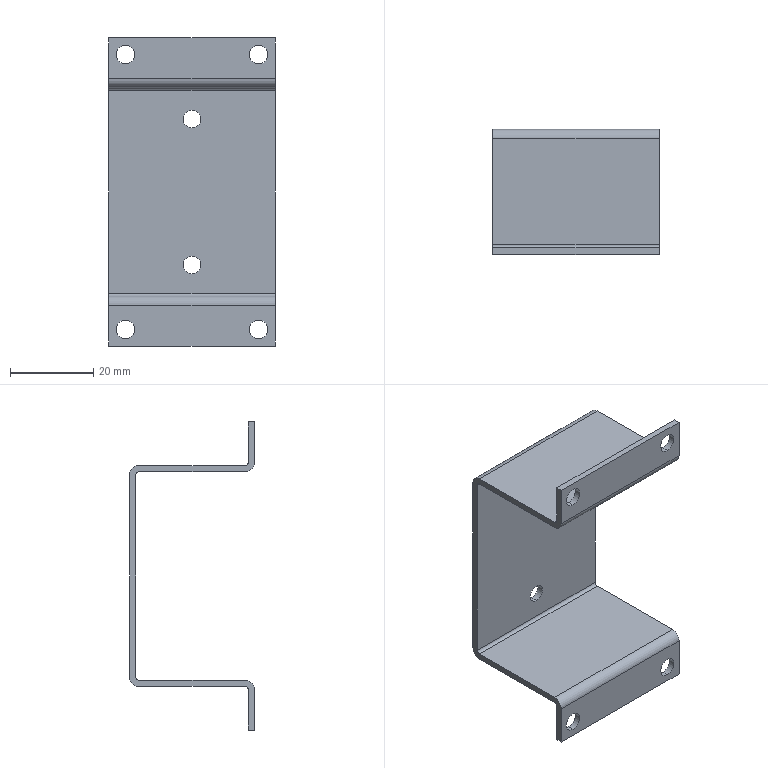Part | SolidWorks | features BaseBody 1 | 1 solid | 34 faces | box 40 x 30 x 74 mm | volume 7570 mm3 | cylinder 20 | plane 14 | commonest cylinder face diameters 4.5 x8 1.473 x4 4.2 x4 4.473 x4
STEP:
#1=CARTESIAN_POINT('',(0.,28.5,19.6));
#2=VERTEX_POINT('',#1);
#3=CARTESIAN_POINT('',(0.,28.5,15.4));
#4=VERTEX_POINT('',#3);
#5=CARTESIAN_POINT('',(0.,28.5,17.5));
#6=DIRECTION('',(0.,-1.,0.));
#7=DIRECTION('',(0.,0.,-1.));
#8=AXIS2_PLACEMENT_3D('',#5,#6,#7);
#9=CIRCLE('',#8,2.1);
#10=EDGE_CURVE('',#2,#4,#9,.T.);
#11=ORIENTED_EDGE('',*,*,#10,.T.);
#12=CARTESIAN_POINT('',(0.,30.,15.4));
#13=VERTEX_POINT('',#12);
#14=CARTESIAN_POINT('',(0.,30.,15.4));
#15=DIRECTION('',(0.,1.,0.));
#16=VECTOR('',#15,1000.);
#17=LINE('',#14,#16);
#18=EDGE_CURVE('',#4,#13,#17,.T.);
#19=ORIENTED_EDGE('',*,*,#18,.T.);
#20=CARTESIAN_POINT('',(0.,30.,19.6));
#21=VERTEX_POINT('',#20);
#22=CARTESIAN_POINT('',(0.,30.,17.5));
#23=DIRECTION('',(0.,1.,0.));
#24=DIRECTION('',(0.,0.,1.));
#25=AXIS2_PLACEMENT_3D('',#22,#23,#24);
#26=CIRCLE('',#25,2.1);
#27=EDGE_CURVE('',#13,#21,#26,.T.);
#28=ORIENTED_EDGE('',*,*,#27,.T.);
#29=CARTESIAN_POINT('',(0.,30.,19.6));
#30=DIRECTION('',(0.,1.,0.));
#31=VECTOR('',#30,1000.);
#32=LINE('',#29,#31);
#33=EDGE_CURVE('',#2,#21,#32,.T.);
#34=ORIENTED_EDGE('',*,*,#33,.F.);
#35=EDGE_LOOP('',(#11,#19,#28,#34));
#36=FACE_OUTER_BOUND('',#35,.T.);
#37=CARTESIAN_POINT('',(0.,30.,17.5));
#38=DIRECTION('',(0.,1.,0.));
#39=DIRECTION('',(0.,0.,1.));
#40=AXIS2_PLACEMENT_3D('',#37,#38,#39);
#41=CYLINDRICAL_SURFACE('',#40,2.1);
#42=ADVANCED_FACE('',(#36),#41,.F.);
#43=CARTESIAN_POINT('',(0.,28.5,-15.4));
#44=VERTEX_POINT('',#43);
#45=CARTESIAN_POINT('',(0.,28.5,-19.6));
#46=VERTEX_POINT('',#45);
#47=CARTESIAN_POINT('',(0.,28.5,-17.5));
#48=DIRECTION('',(0.,-1.,0.));
#49=DIRECTION('',(0.,0.,-1.));
#50=AXIS2_PLACEMENT_3D('',#47,#48,#49);
#51=CIRCLE('',#50,2.1);
#52=EDGE_CURVE('',#44,#46,#51,.T.);
#53=ORIENTED_EDGE('',*,*,#52,.T.);
#54=CARTESIAN_POINT('',(0.,30.,-19.6));
#55=VERTEX_POINT('',#54);
#56=CARTESIAN_POINT('',(0.,30.,-19.6));
#57=DIRECTION('',(0.,1.,0.));
#58=VECTOR('',#57,1000.);
#59=LINE('',#56,#58);
#60=EDGE_CURVE('',#46,#55,#59,.T.);
#61=ORIENTED_EDGE('',*,*,#60,.T.);
#62=CARTESIAN_POINT('',(0.,30.,-15.4));
#63=VERTEX_POINT('',#62);
#64=CARTESIAN_POINT('',(0.,30.,-17.5));
#65=DIRECTION('',(0.,1.,0.));
#66=DIRECTION('',(0.,0.,1.));
#67=AXIS2_PLACEMENT_3D('',#64,#65,#66);
#68=CIRCLE('',#67,2.1);
#69=EDGE_CURVE('',#55,#63,#68,.T.);
#70=ORIENTED_EDGE('',*,*,#69,.T.);
#71=CARTESIAN_POINT('',(0.,30.,-15.4));
#72=DIRECTION('',(0.,1.,0.));
#73=VECTOR('',#72,1000.);
#74=LINE('',#71,#73);
#75=EDGE_CURVE('',#44,#63,#74,.T.);
#76=ORIENTED_EDGE('',*,*,#75,.F.);
#77=EDGE_LOOP('',(#53,#61,#70,#76));
#78=FACE_OUTER_BOUND('',#77,.T.);
#79=CARTESIAN_POINT('',(0.,30.,-17.5));
#80=DIRECTION('',(0.,1.,0.));
#81=DIRECTION('',(0.,0.,1.));
#82=AXIS2_PLACEMENT_3D('',#79,#80,#81);
#83=CYLINDRICAL_SURFACE('',#82,2.1);
#84=ADVANCED_FACE('',(#78),#83,.F.);
#85=CARTESIAN_POINT('',(-16.,0.,30.75));
#86=VERTEX_POINT('',#85);
#87=CARTESIAN_POINT('',(-16.,0.,35.25));
#88=VERTEX_POINT('',#87);
#89=CARTESIAN_POINT('',(-16.,0.,33.));
#90=DIRECTION('',(0.,1.,0.));
#91=DIRECTION('',(0.,0.,-1.));
#92=AXIS2_PLACEMENT_3D('',#89,#90,#91);
#93=CIRCLE('',#92,2.25);
#94=EDGE_CURVE('',#86,#88,#93,.T.);
#95=ORIENTED_EDGE('',*,*,#94,.F.);
#96=CARTESIAN_POINT('',(-16.,1.5,30.75));
#97=VERTEX_POINT('',#96);
#98=CARTESIAN_POINT('',(-16.,0.,30.75));
#99=DIRECTION('',(0.,1.,0.));
#100=VECTOR('',#99,1000.);
#101=LINE('',#98,#100);
#102=EDGE_CURVE('',#86,#97,#101,.T.);
#103=ORIENTED_EDGE('',*,*,#102,.T.);
#104=CARTESIAN_POINT('',(-16.,1.5,35.25));
#105=VERTEX_POINT('',#104);
#106=CARTESIAN_POINT('',(-16.,1.5,33.));
#107=DIRECTION('',(0.,1.,0.));
#108=DIRECTION('',(0.,0.,-1.));
#109=AXIS2_PLACEMENT_3D('',#106,#107,#108);
#110=CIRCLE('',#109,2.25);
#111=EDGE_CURVE('',#97,#105,#110,.T.);
#112=ORIENTED_EDGE('',*,*,#111,.T.);
#113=CARTESIAN_POINT('',(-16.,0.,35.25));
#114=DIRECTION('',(0.,1.,0.));
#115=VECTOR('',#114,1000.);
#116=LINE('',#113,#115);
#117=EDGE_CURVE('',#88,#105,#116,.T.);
#118=ORIENTED_EDGE('',*,*,#117,.F.);
#119=EDGE_LOOP('',(#95,#103,#112,#118));
#120=FACE_OUTER_BOUND('',#119,.T.);
#121=CARTESIAN_POINT('',(-16.,0.,33.));
#122=DIRECTION('',(0.,1.,0.));
#123=DIRECTION('',(0.,0.,1.));
#124=AXIS2_PLACEMENT_3D('',#121,#122,#123);
#125=CYLINDRICAL_SURFACE('',#124,2.25);
#126=ADVANCED_FACE('',(#120),#125,.F.);
#127=CARTESIAN_POINT('',(16.,0.,30.75));
#128=VERTEX_POINT('',#127);
#129=CARTESIAN_POINT('',(16.,0.,35.25));
#130=VERTEX_POINT('',#129);
#131=CARTESIAN_POINT('',(16.,0.,33.));
#132=DIRECTION('',(0.,1.,0.));
#133=DIRECTION('',(0.,0.,1.));
#134=AXIS2_PLACEMENT_3D('',#131,#132,#133);
#135=CIRCLE('',#134,2.25);
#136=EDGE_CURVE('',#128,#130,#135,.T.);
#137=ORIENTED_EDGE('',*,*,#136,.F.);
#138=CARTESIAN_POINT('',(16.,1.5,30.75));
#139=VERTEX_POINT('',#138);
#140=CARTESIAN_POINT('',(16.,0.,30.75));
#141=DIRECTION('',(0.,1.,0.));
#142=VECTOR('',#141,1000.);
#143=LINE('',#140,#142);
#144=EDGE_CURVE('',#128,#139,#143,.T.);
#145=ORIENTED_EDGE('',*,*,#144,.T.);
#146=CARTESIAN_POINT('',(16.,1.5,35.25));
#147=VERTEX_POINT('',#146);
#148=CARTESIAN_POINT('',(16.,1.5,33.));
#149=DIRECTION('',(0.,1.,0.));
#150=DIRECTION('',(0.,0.,1.));
#151=AXIS2_PLACEMENT_3D('',#148,#149,#150);
#152=CIRCLE('',#151,2.25);
#153=EDGE_CURVE('',#139,#147,#152,.T.);
#154=ORIENTED_EDGE('',*,*,#153,.T.);
#155=CARTESIAN_POINT('',(16.,0.,35.25));
#156=DIRECTION('',(0.,1.,0.));
#157=VECTOR('',#156,1000.);
#158=LINE('',#155,#157);
#159=EDGE_CURVE('',#130,#147,#158,.T.);
#160=ORIENTED_EDGE('',*,*,#159,.F.);
#161=EDGE_LOOP('',(#137,#145,#154,#160));
#162=FACE_OUTER_BOUND('',#161,.T.);
#163=CARTESIAN_POINT('',(16.,0.,33.));
#164=DIRECTION('',(0.,1.,0.));
#165=DIRECTION('',(0.,0.,1.));
#166=AXIS2_PLACEMENT_3D('',#163,#164,#165);
#167=CYLINDRICAL_SURFACE('',#166,2.25);
#168=ADVANCED_FACE('',(#162),#167,.F.);
#169=CARTESIAN_POINT('',(16.,0.,-35.25));
#170=VERTEX_POINT('',#169);
#171=CARTESIAN_POINT('',(16.,0.,-30.75));
#172=VERTEX_POINT('',#171);
#173=CARTESIAN_POINT('',(16.,0.,-33.));
#174=DIRECTION('',(0.,1.,0.));
#175=DIRECTION('',(0.,0.,-1.));
#176=AXIS2_PLACEMENT_3D('',#173,#174,#175);
#177=CIRCLE('',#176,2.25);
#178=EDGE_CURVE('',#170,#172,#177,.T.);
#179=ORIENTED_EDGE('',*,*,#178,.F.);
#180=CARTESIAN_POINT('',(16.,1.5,-35.25));
#181=VERTEX_POINT('',#180);
#182=CARTESIAN_POINT('',(16.,0.,-35.25));
#183=DIRECTION('',(0.,1.,0.));
#184=VECTOR('',#183,1000.);
#185=LINE('',#182,#184);
#186=EDGE_CURVE('',#170,#181,#185,.T.);
#187=ORIENTED_EDGE('',*,*,#186,.T.);
#188=CARTESIAN_POINT('',(16.,1.5,-30.75));
#189=VERTEX_POINT('',#188);
#190=CARTESIAN_POINT('',(16.,1.5,-33.));
#191=DIRECTION('',(0.,1.,0.));
#192=DIRECTION('',(0.,0.,-1.));
#193=AXIS2_PLACEMENT_3D('',#190,#191,#192);
#194=CIRCLE('',#193,2.25);
#195=EDGE_CURVE('',#181,#189,#194,.T.);
#196=ORIENTED_EDGE('',*,*,#195,.T.);
#197=CARTESIAN_POINT('',(16.,0.,-30.75));
#198=DIRECTION('',(0.,1.,0.));
#199=VECTOR('',#198,1000.);
#200=LINE('',#197,#199);
#201=EDGE_CURVE('',#172,#189,#200,.T.);
#202=ORIENTED_EDGE('',*,*,#201,.F.);
#203=EDGE_LOOP('',(#179,#187,#196,#202));
#204=FACE_OUTER_BOUND('',#203,.T.);
#205=CARTESIAN_POINT('',(16.,0.,-33.));
#206=DIRECTION('',(0.,1.,0.));
#207=DIRECTION('',(0.,0.,1.));
#208=AXIS2_PLACEMENT_3D('',#205,#206,#207);
#209=CYLINDRICAL_SURFACE('',#208,2.25);
#210=ADVANCED_FACE('',(#204),#209,.F.);
#211=CARTESIAN_POINT('',(-16.,0.,-35.25));
#212=VERTEX_POINT('',#211);
#213=CARTESIAN_POINT('',(-16.,0.,-30.75));
#214=VERTEX_POINT('',#213);
#215=CARTESIAN_POINT('',(-16.,0.,-33.));
#216=DIRECTION('',(0.,1.,0.));
#217=DIRECTION('',(0.,0.,1.));
#218=AXIS2_PLACEMENT_3D('',#215,#216,#217);
#219=CIRCLE('',#218,2.25);
#220=EDGE_CURVE('',#212,#214,#219,.T.);
#221=ORIENTED_EDGE('',*,*,#220,.F.);
#222=CARTESIAN_POINT('',(-16.,1.5,-35.25));
#223=VERTEX_POINT('',#222);
#224=CARTESIAN_POINT('',(-16.,0.,-35.25));
#225=DIRECTION('',(0.,1.,0.));
#226=VECTOR('',#225,1000.);
#227=LINE('',#224,#226);
#228=EDGE_CURVE('',#212,#223,#227,.T.);
#229=ORIENTED_EDGE('',*,*,#228,.T.);
#230=CARTESIAN_POINT('',(-16.,1.5,-30.75));
#231=VERTEX_POINT('',#230);
#232=CARTESIAN_POINT('',(-16.,1.5,-33.));
#233=DIRECTION('',(0.,1.,0.));
#234=DIRECTION('',(0.,0.,1.));
#235=AXIS2_PLACEMENT_3D('',#232,#233,#234);
#236=CIRCLE('',#235,2.25);
#237=EDGE_CURVE('',#223,#231,#236,.T.);
#238=ORIENTED_EDGE('',*,*,#237,.T.);
#239=CARTESIAN_POINT('',(-16.,0.,-30.75));
#240=DIRECTION('',(0.,1.,0.));
#241=VECTOR('',#240,1000.);
#242=LINE('',#239,#241);
#243=EDGE_CURVE('',#214,#231,#242,.T.);
#244=ORIENTED_EDGE('',*,*,#243,.F.);
#245=EDGE_LOOP('',(#221,#229,#238,#244));
#246=FACE_OUTER_BOUND('',#245,.T.);
#247=CARTESIAN_POINT('',(-16.,0.,-33.));
#248=DIRECTION('',(0.,1.,0.));
#249=DIRECTION('',(0.,0.,1.));
#250=AXIS2_PLACEMENT_3D('',#247,#248,#249);
#251=CYLINDRICAL_SURFACE('',#250,2.25);
#252=ADVANCED_FACE('',(#246),#251,.F.);
#253=CARTESIAN_POINT('',(-20.,2.237,26.5));
#254=VERTEX_POINT('',#253);
#255=CARTESIAN_POINT('',(-20.,1.5,27.237));
#256=VERTEX_POINT('',#255);
#257=CARTESIAN_POINT('',(-20.,2.237,27.237));
#258=DIRECTION('',(-1.,0.,0.));
#259=DIRECTION('',(0.,0.,-1.));
#260=AXIS2_PLACEMENT_3D('',#257,#258,#259);
#261=CIRCLE('',#260,0.7366);
#262=EDGE_CURVE('',#254,#256,#261,.T.);
#263=ORIENTED_EDGE('',*,*,#262,.T.);
#264=CARTESIAN_POINT('',(20.,1.5,27.237));
#265=VERTEX_POINT('',#264);
#266=CARTESIAN_POINT('',(20.,1.5,27.237));
#267=DIRECTION('',(-1.,0.,0.));
#268=VECTOR('',#267,1000.);
#269=LINE('',#266,#268);
#270=EDGE_CURVE('',#265,#256,#269,.T.);
#271=ORIENTED_EDGE('',*,*,#270,.F.);
#272=CARTESIAN_POINT('',(20.,2.237,26.5));
#273=VERTEX_POINT('',#272);
#274=CARTESIAN_POINT('',(20.,2.237,27.237));
#275=DIRECTION('',(-1.,0.,0.));
#276=DIRECTION('',(0.,0.,-1.));
#277=AXIS2_PLACEMENT_3D('',#274,#275,#276);
#278=CIRCLE('',#277,0.7366);
#279=EDGE_CURVE('',#273,#265,#278,.T.);
#280=ORIENTED_EDGE('',*,*,#279,.F.);
#281=CARTESIAN_POINT('',(20.,2.237,26.5));
#282=DIRECTION('',(-1.,0.,0.));
#283=VECTOR('',#282,1000.);
#284=LINE('',#281,#283);
#285=EDGE_CURVE('',#273,#254,#284,.T.);
#286=ORIENTED_EDGE('',*,*,#285,.T.);
#287=EDGE_LOOP('',(#263,#271,#280,#286));
#288=FACE_OUTER_BOUND('',#287,.T.);
#289=CARTESIAN_POINT('',(20.,2.237,27.237));
#290=DIRECTION('',(-1.,0.,0.));
#291=DIRECTION('',(0.,0.,1.));
#292=AXIS2_PLACEMENT_3D('',#289,#290,#291);
#293=CYLINDRICAL_SURFACE('',#292,0.7366);
#294=ADVANCED_FACE('',(#288),#293,.F.);
#295=CARTESIAN_POINT('',(-20.,27.763,26.5));
#296=VERTEX_POINT('',#295);
#297=CARTESIAN_POINT('',(-20.,0.,26.5));
#298=DIRECTION('',(0.,-1.,0.));
#299=VECTOR('',#298,1000.);
#300=LINE('',#297,#299);
#301=EDGE_CURVE('',#296,#254,#300,.T.);
#302=ORIENTED_EDGE('',*,*,#301,.T.);
#303=ORIENTED_EDGE('',*,*,#285,.F.);
#304=CARTESIAN_POINT('',(20.,27.763,26.5));
#305=VERTEX_POINT('',#304);
#306=CARTESIAN_POINT('',(20.,0.,26.5));
#307=DIRECTION('',(0.,-1.,0.));
#308=VECTOR('',#307,1000.);
#309=LINE('',#306,#308);
#310=EDGE_CURVE('',#305,#273,#309,.T.);
#311=ORIENTED_EDGE('',*,*,#310,.F.);
#312=CARTESIAN_POINT('',(20.,27.763,26.5));
#313=DIRECTION('',(-1.,0.,0.));
#314=VECTOR('',#313,1000.);
#315=LINE('',#312,#314);
#316=EDGE_CURVE('',#305,#296,#315,.T.);
#317=ORIENTED_EDGE('',*,*,#316,.T.);
#318=EDGE_LOOP('',(#302,#303,#311,#317));
#319=FACE_OUTER_BOUND('',#318,.T.);
#320=CARTESIAN_POINT('',(20.,0.,26.5));
#321=DIRECTION('',(0.,0.,-1.));
#322=DIRECTION('',(0.,-1.,0.));
#323=AXIS2_PLACEMENT_3D('',#320,#321,#322);
#324=PLANE('',#323);
#325=ADVANCED_FACE('',(#319),#324,.F.);
#326=CARTESIAN_POINT('',(-20.,30.,24.263));
#327=VERTEX_POINT('',#326);
#328=CARTESIAN_POINT('',(-20.,27.763,24.263));
#329=DIRECTION('',(1.,0.,0.));
#330=DIRECTION('',(0.,0.,-1.));
#331=AXIS2_PLACEMENT_3D('',#328,#329,#330);
#332=CIRCLE('',#331,2.237);
#333=EDGE_CURVE('',#327,#296,#332,.T.);
#334=ORIENTED_EDGE('',*,*,#333,.T.);
#335=ORIENTED_EDGE('',*,*,#316,.F.);
#336=CARTESIAN_POINT('',(20.,30.,24.263));
#337=VERTEX_POINT('',#336);
#338=CARTESIAN_POINT('',(20.,27.763,24.263));
#339=DIRECTION('',(1.,0.,0.));
#340=DIRECTION('',(0.,0.,-1.));
#341=AXIS2_PLACEMENT_3D('',#338,#339,#340);
#342=CIRCLE('',#341,2.237);
#343=EDGE_CURVE('',#337,#305,#342,.T.);
#344=ORIENTED_EDGE('',*,*,#343,.F.);
#345=CARTESIAN_POINT('',(20.,30.,24.263));
#346=DIRECTION('',(-1.,0.,0.));
#347=VECTOR('',#346,1000.);
#348=LINE('',#345,#347);
#349=EDGE_CURVE('',#337,#327,#348,.T.);
#350=ORIENTED_EDGE('',*,*,#349,.T.);
#351=EDGE_LOOP('',(#334,#335,#344,#350));
#352=FACE_OUTER_BOUND('',#351,.T.);
#353=CARTESIAN_POINT('',(20.,27.763,24.263));
#354=DIRECTION('',(-1.,0.,0.));
#355=DIRECTION('',(0.,0.,1.));
#356=AXIS2_PLACEMENT_3D('',#353,#354,#355);
#357=CYLINDRICAL_SURFACE('',#356,2.237);
#358=ADVANCED_FACE('',(#352),#357,.T.);
#359=CARTESIAN_POINT('',(-20.,27.763,-26.5));
#360=VERTEX_POINT('',#359);
#361=CARTESIAN_POINT('',(-20.,30.,-24.263));
#362=VERTEX_POINT('',#361);
#363=CARTESIAN_POINT('',(-20.,27.763,-24.263));
#364=DIRECTION('',(1.,0.,0.));
#365=DIRECTION('',(0.,0.,-1.));
#366=AXIS2_PLACEMENT_3D('',#363,#364,#365);
#367=CIRCLE('',#366,2.237);
#368=EDGE_CURVE('',#360,#362,#367,.T.);
#369=ORIENTED_EDGE('',*,*,#368,.T.);
#370=CARTESIAN_POINT('',(20.,30.,-24.263));
#371=VERTEX_POINT('',#370);
#372=CARTESIAN_POINT('',(20.,30.,-24.263));
#373=DIRECTION('',(-1.,0.,0.));
#374=VECTOR('',#373,1000.);
#375=LINE('',#372,#374);
#376=EDGE_CURVE('',#371,#362,#375,.T.);
#377=ORIENTED_EDGE('',*,*,#376,.F.);
#378=CARTESIAN_POINT('',(20.,27.763,-26.5));
#379=VERTEX_POINT('',#378);
#380=CARTESIAN_POINT('',(20.,27.763,-24.263));
#381=DIRECTION('',(1.,0.,0.));
#382=DIRECTION('',(0.,0.,-1.));
#383=AXIS2_PLACEMENT_3D('',#380,#381,#382);
#384=CIRCLE('',#383,2.237);
#385=EDGE_CURVE('',#379,#371,#384,.T.);
#386=ORIENTED_EDGE('',*,*,#385,.F.);
#387=CARTESIAN_POINT('',(20.,27.763,-26.5));
#388=DIRECTION('',(-1.,0.,0.));
#389=VECTOR('',#388,1000.);
#390=LINE('',#387,#389);
#391=EDGE_CURVE('',#379,#360,#390,.T.);
#392=ORIENTED_EDGE('',*,*,#391,.T.);
#393=EDGE_LOOP('',(#369,#377,#386,#392));
#394=FACE_OUTER_BOUND('',#393,.T.);
#395=CARTESIAN_POINT('',(20.,27.763,-24.263));
#396=DIRECTION('',(-1.,0.,0.));
#397=DIRECTION('',(0.,0.,1.));
#398=AXIS2_PLACEMENT_3D('',#395,#396,#397);
#399=CYLINDRICAL_SURFACE('',#398,2.237);
#400=ADVANCED_FACE('',(#394),#399,.T.);
#401=CARTESIAN_POINT('',(-20.,2.237,-26.5));
#402=VERTEX_POINT('',#401);
#403=CARTESIAN_POINT('',(-20.,0.,-26.5));
#404=DIRECTION('',(0.,1.,0.));
#405=VECTOR('',#404,1000.);
#406=LINE('',#403,#405);
#407=EDGE_CURVE('',#402,#360,#406,.T.);
#408=ORIENTED_EDGE('',*,*,#407,.T.);
#409=ORIENTED_EDGE('',*,*,#391,.F.);
#410=CARTESIAN_POINT('',(20.,2.237,-26.5));
#411=VERTEX_POINT('',#410);
#412=CARTESIAN_POINT('',(20.,0.,-26.5));
#413=DIRECTION('',(0.,1.,0.));
#414=VECTOR('',#413,1000.);
#415=LINE('',#412,#414);
#416=EDGE_CURVE('',#411,#379,#415,.T.);
#417=ORIENTED_EDGE('',*,*,#416,.F.);
#418=CARTESIAN_POINT('',(20.,2.237,-26.5));
#419=DIRECTION('',(-1.,0.,0.));
#420=VECTOR('',#419,1000.);
#421=LINE('',#418,#420);
#422=EDGE_CURVE('',#411,#402,#421,.T.);
#423=ORIENTED_EDGE('',*,*,#422,.T.);
#424=EDGE_LOOP('',(#408,#409,#417,#423));
#425=FACE_OUTER_BOUND('',#424,.T.);
#426=CARTESIAN_POINT('',(20.,0.,-26.5));
#427=DIRECTION('',(0.,0.,1.));
#428=DIRECTION('',(1.,0.,0.));
#429=AXIS2_PLACEMENT_3D('',#426,#427,#428);
#430=PLANE('',#429);
#431=ADVANCED_FACE('',(#425),#430,.F.);
#432=CARTESIAN_POINT('',(-20.,1.5,-27.237));
#433=VERTEX_POINT('',#432);
#434=CARTESIAN_POINT('',(-20.,2.237,-27.237));
#435=DIRECTION('',(-1.,0.,0.));
#436=DIRECTION('',(0.,0.,-1.));
#437=AXIS2_PLACEMENT_3D('',#434,#435,#436);
#438=CIRCLE('',#437,0.7366);
#439=EDGE_CURVE('',#433,#402,#438,.T.);
#440=ORIENTED_EDGE('',*,*,#439,.T.);
#441=ORIENTED_EDGE('',*,*,#422,.F.);
#442=CARTESIAN_POINT('',(20.,1.5,-27.237));
#443=VERTEX_POINT('',#442);
#444=CARTESIAN_POINT('',(20.,2.237,-27.237));
#445=DIRECTION('',(-1.,0.,0.));
#446=DIRECTION('',(0.,0.,-1.));
#447=AXIS2_PLACEMENT_3D('',#444,#445,#446);
#448=CIRCLE('',#447,0.7366);
#449=EDGE_CURVE('',#443,#411,#448,.T.);
#450=ORIENTED_EDGE('',*,*,#449,.F.);
#451=CARTESIAN_POINT('',(20.,1.5,-27.237));
#452=DIRECTION('',(-1.,0.,0.));
#453=VECTOR('',#452,1000.);
#454=LINE('',#451,#453);
#455=EDGE_CURVE('',#443,#433,#454,.T.);
#456=ORIENTED_EDGE('',*,*,#455,.T.);
#457=EDGE_LOOP('',(#440,#441,#450,#456));
#458=FACE_OUTER_BOUND('',#457,.T.);
#459=CARTESIAN_POINT('',(20.,2.237,-27.237));
#460=DIRECTION('',(-1.,0.,0.));
#461=DIRECTION('',(0.,0.,1.));
#462=AXIS2_PLACEMENT_3D('',#459,#460,#461);
#463=CYLINDRICAL_SURFACE('',#462,0.7366);
#464=ADVANCED_FACE('',(#458),#463,.F.);
#465=CARTESIAN_POINT('',(-16.,1.5,-33.));
#466=DIRECTION('',(0.,1.,0.));
#467=DIRECTION('',(0.,0.,1.));
#468=AXIS2_PLACEMENT_3D('',#465,#466,#467);
#469=CIRCLE('',#468,2.25);
#470=EDGE_CURVE('',#231,#223,#469,.T.);
#471=ORIENTED_EDGE('',*,*,#470,.F.);
#472=ORIENTED_EDGE('',*,*,#237,.F.);
#473=EDGE_LOOP('',(#471,#472));
#474=FACE_BOUND('',#473,.T.);
#475=CARTESIAN_POINT('',(16.,1.5,-33.));
#476=DIRECTION('',(0.,1.,0.));
#477=DIRECTION('',(0.,0.,-1.));
#478=AXIS2_PLACEMENT_3D('',#475,#476,#477);
#479=CIRCLE('',#478,2.25);
#480=EDGE_CURVE('',#189,#181,#479,.T.);
#481=ORIENTED_EDGE('',*,*,#480,.F.);
#482=ORIENTED_EDGE('',*,*,#195,.F.);
#483=EDGE_LOOP('',(#481,#482));
#484=FACE_BOUND('',#483,.T.);
#485=CARTESIAN_POINT('',(-20.,1.5,-37.));
#486=VERTEX_POINT('',#485);
#487=CARTESIAN_POINT('',(-20.,1.5,-37.));
#488=DIRECTION('',(0.,0.,1.));
#489=VECTOR('',#488,1000.);
#490=LINE('',#487,#489);
#491=EDGE_CURVE('',#486,#433,#490,.T.);
#492=ORIENTED_EDGE('',*,*,#491,.T.);
#493=ORIENTED_EDGE('',*,*,#455,.F.);
#494=CARTESIAN_POINT('',(20.,1.5,-37.));
#495=VERTEX_POINT('',#494);
#496=CARTESIAN_POINT('',(20.,1.5,-37.));
#497=DIRECTION('',(0.,0.,1.));
#498=VECTOR('',#497,1000.);
#499=LINE('',#496,#498);
#500=EDGE_CURVE('',#495,#443,#499,.T.);
#501=ORIENTED_EDGE('',*,*,#500,.F.);
#502=CARTESIAN_POINT('',(20.,1.5,-37.));
#503=DIRECTION('',(-1.,0.,0.));
#504=VECTOR('',#503,1000.);
#505=LINE('',#502,#504);
#506=EDGE_CURVE('',#495,#486,#505,.T.);
#507=ORIENTED_EDGE('',*,*,#506,.T.);
#508=EDGE_LOOP('',(#492,#493,#501,#507));
#509=FACE_OUTER_BOUND('',#508,.T.);
#510=CARTESIAN_POINT('',(20.,1.5,-37.));
#511=DIRECTION('',(0.,-1.,0.));
#512=DIRECTION('',(-1.,0.,0.));
#513=AXIS2_PLACEMENT_3D('',#510,#511,#512);
#514=PLANE('',#513);
#515=ADVANCED_FACE('',(#474,#484,#509),#514,.F.);
#516=CARTESIAN_POINT('',(-20.,0.,-37.));
#517=VERTEX_POINT('',#516);
#518=CARTESIAN_POINT('',(-20.,1.5,-37.));
#519=DIRECTION('',(0.,-1.,0.));
#520=VECTOR('',#519,1000.);
#521=LINE('',#518,#520);
#522=EDGE_CURVE('',#486,#517,#521,.T.);
#523=ORIENTED_EDGE('',*,*,#522,.F.);
#524=ORIENTED_EDGE('',*,*,#506,.F.);
#525=CARTESIAN_POINT('',(20.,0.,-37.));
#526=VERTEX_POINT('',#525);
#527=CARTESIAN_POINT('',(20.,1.5,-37.));
#528=DIRECTION('',(0.,-1.,0.));
#529=VECTOR('',#528,1000.);
#530=LINE('',#527,#529);
#531=EDGE_CURVE('',#495,#526,#530,.T.);
#532=ORIENTED_EDGE('',*,*,#531,.T.);
#533=CARTESIAN_POINT('',(20.,0.,-37.));
#534=DIRECTION('',(-1.,0.,0.));
#535=VECTOR('',#534,1000.);
#536=LINE('',#533,#535);
#537=EDGE_CURVE('',#526,#517,#536,.T.);
#538=ORIENTED_EDGE('',*,*,#537,.T.);
#539=EDGE_LOOP('',(#523,#524,#532,#538));
#540=FACE_OUTER_BOUND('',#539,.T.);
#541=CARTESIAN_POINT('',(20.,1.5,-37.));
#542=DIRECTION('',(0.,0.,-1.));
#543=DIRECTION('',(0.,-1.,0.));
#544=AXIS2_PLACEMENT_3D('',#541,#542,#543);
#545=PLANE('',#544);
#546=ADVANCED_FACE('',(#540),#545,.T.);
#547=CARTESIAN_POINT('',(-16.,0.,-33.));
#548=DIRECTION('',(0.,1.,0.));
#549=DIRECTION('',(0.,0.,1.));
#550=AXIS2_PLACEMENT_3D('',#547,#548,#549);
#551=CIRCLE('',#550,2.25);
#552=EDGE_CURVE('',#214,#212,#551,.T.);
#553=ORIENTED_EDGE('',*,*,#552,.T.);
#554=ORIENTED_EDGE('',*,*,#220,.T.);
#555=EDGE_LOOP('',(#553,#554));
#556=FACE_BOUND('',#555,.T.);
#557=CARTESIAN_POINT('',(16.,0.,-33.));
#558=DIRECTION('',(0.,1.,0.));
#559=DIRECTION('',(0.,0.,-1.));
#560=AXIS2_PLACEMENT_3D('',#557,#558,#559);
#561=CIRCLE('',#560,2.25);
#562=EDGE_CURVE('',#172,#170,#561,.T.);
#563=ORIENTED_EDGE('',*,*,#562,.T.);
#564=ORIENTED_EDGE('',*,*,#178,.T.);
#565=EDGE_LOOP('',(#563,#564));
#566=FACE_BOUND('',#565,.T.);
#567=CARTESIAN_POINT('',(-20.,0.,-27.237));
#568=VERTEX_POINT('',#567);
#569=CARTESIAN_POINT('',(-20.,0.,-37.));
#570=DIRECTION('',(0.,0.,1.));
#571=VECTOR('',#570,1000.);
#572=LINE('',#569,#571);
#573=EDGE_CURVE('',#517,#568,#572,.T.);
#574=ORIENTED_EDGE('',*,*,#573,.F.);
#575=ORIENTED_EDGE('',*,*,#537,.F.);
#576=CARTESIAN_POINT('',(20.,0.,-27.237));
#577=VERTEX_POINT('',#576);
#578=CARTESIAN_POINT('',(20.,0.,-37.));
#579=DIRECTION('',(0.,0.,1.));
#580=VECTOR('',#579,1000.);
#581=LINE('',#578,#580);
#582=EDGE_CURVE('',#526,#577,#581,.T.);
#583=ORIENTED_EDGE('',*,*,#582,.T.);
#584=CARTESIAN_POINT('',(20.,0.,-27.237));
#585=DIRECTION('',(-1.,0.,0.));
#586=VECTOR('',#585,1000.);
#587=LINE('',#584,#586);
#588=EDGE_CURVE('',#577,#568,#587,.T.);
#589=ORIENTED_EDGE('',*,*,#588,.T.);
#590=EDGE_LOOP('',(#574,#575,#583,#589));
#591=FACE_OUTER_BOUND('',#590,.T.);
#592=CARTESIAN_POINT('',(20.,0.,-37.));
#593=DIRECTION('',(0.,-1.,0.));
#594=DIRECTION('',(-1.,0.,0.));
#595=AXIS2_PLACEMENT_3D('',#592,#593,#594);
#596=PLANE('',#595);
#597=ADVANCED_FACE('',(#556,#566,#591),#596,.T.);
#598=CARTESIAN_POINT('',(-20.,2.237,-25.));
#599=VERTEX_POINT('',#598);
#600=CARTESIAN_POINT('',(-20.,2.237,-27.237));
#601=DIRECTION('',(-1.,0.,0.));
#602=DIRECTION('',(0.,0.,1.));
#603=AXIS2_PLACEMENT_3D('',#600,#601,#602);
#604=CIRCLE('',#603,2.237);
#605=EDGE_CURVE('',#568,#599,#604,.T.);
#606=ORIENTED_EDGE('',*,*,#605,.F.);
#607=ORIENTED_EDGE('',*,*,#588,.F.);
#608=CARTESIAN_POINT('',(20.,2.237,-25.));
#609=VERTEX_POINT('',#608);
#610=CARTESIAN_POINT('',(20.,2.237,-27.237));
#611=DIRECTION('',(-1.,0.,0.));
#612=DIRECTION('',(0.,0.,1.));
#613=AXIS2_PLACEMENT_3D('',#610,#611,#612);
#614=CIRCLE('',#613,2.237);
#615=EDGE_CURVE('',#577,#609,#614,.T.);
#616=ORIENTED_EDGE('',*,*,#615,.T.);
#617=CARTESIAN_POINT('',(20.,2.237,-25.));
#618=DIRECTION('',(-1.,0.,0.));
#619=VECTOR('',#618,1000.);
#620=LINE('',#617,#619);
#621=EDGE_CURVE('',#609,#599,#620,.T.);
#622=ORIENTED_EDGE('',*,*,#621,.T.);
#623=EDGE_LOOP('',(#606,#607,#616,#622));
#624=FACE_OUTER_BOUND('',#623,.T.);
#625=CARTESIAN_POINT('',(20.,2.237,-27.237));
#626=DIRECTION('',(-1.,0.,0.));
#627=DIRECTION('',(0.,0.,1.));
#628=AXIS2_PLACEMENT_3D('',#625,#626,#627);
#629=CYLINDRICAL_SURFACE('',#628,2.237);
#630=ADVANCED_FACE('',(#624),#629,.T.);
#631=CARTESIAN_POINT('',(-20.,27.763,-25.));
#632=VERTEX_POINT('',#631);
#633=CARTESIAN_POINT('',(-20.,0.,-25.));
#634=DIRECTION('',(0.,1.,0.));
#635=VECTOR('',#634,1000.);
#636=LINE('',#633,#635);
#637=EDGE_CURVE('',#599,#632,#636,.T.);
#638=ORIENTED_EDGE('',*,*,#637,.F.);
#639=ORIENTED_EDGE('',*,*,#621,.F.);
#640=CARTESIAN_POINT('',(20.,27.763,-25.));
#641=VERTEX_POINT('',#640);
#642=CARTESIAN_POINT('',(20.,0.,-25.));
#643=DIRECTION('',(0.,1.,0.));
#644=VECTOR('',#643,1000.);
#645=LINE('',#642,#644);
#646=EDGE_CURVE('',#609,#641,#645,.T.);
#647=ORIENTED_EDGE('',*,*,#646,.T.);
#648=CARTESIAN_POINT('',(20.,27.763,-25.));
#649=DIRECTION('',(-1.,0.,0.));
#650=VECTOR('',#649,1000.);
#651=LINE('',#648,#650);
#652=EDGE_CURVE('',#641,#632,#651,.T.);
#653=ORIENTED_EDGE('',*,*,#652,.T.);
#654=EDGE_LOOP('',(#638,#639,#647,#653));
#655=FACE_OUTER_BOUND('',#654,.T.);
#656=CARTESIAN_POINT('',(20.,0.,-25.));
#657=DIRECTION('',(0.,0.,1.));
#658=DIRECTION('',(1.,0.,0.));
#659=AXIS2_PLACEMENT_3D('',#656,#657,#658);
#660=PLANE('',#659);
#661=ADVANCED_FACE('',(#655),#660,.T.);
#662=CARTESIAN_POINT('',(-20.,28.5,-24.263));
#663=VERTEX_POINT('',#662);
#664=CARTESIAN_POINT('',(-20.,27.763,-24.263));
#665=DIRECTION('',(1.,0.,0.));
#666=DIRECTION('',(0.,0.,-1.));
#667=AXIS2_PLACEMENT_3D('',#664,#665,#666);
#668=CIRCLE('',#667,0.7366);
#669=EDGE_CURVE('',#632,#663,#668,.T.);
#670=ORIENTED_EDGE('',*,*,#669,.F.);
#671=ORIENTED_EDGE('',*,*,#652,.F.);
#672=CARTESIAN_POINT('',(20.,28.5,-24.263));
#673=VERTEX_POINT('',#672);
#674=CARTESIAN_POINT('',(20.,27.763,-24.263));
#675=DIRECTION('',(1.,0.,0.));
#676=DIRECTION('',(0.,0.,-1.));
#677=AXIS2_PLACEMENT_3D('',#674,#675,#676);
#678=CIRCLE('',#677,0.7366);
#679=EDGE_CURVE('',#641,#673,#678,.T.);
#680=ORIENTED_EDGE('',*,*,#679,.T.);
#681=CARTESIAN_POINT('',(20.,28.5,-24.263));
#682=DIRECTION('',(-1.,0.,0.));
#683=VECTOR('',#682,1000.);
#684=LINE('',#681,#683);
#685=EDGE_CURVE('',#673,#663,#684,.T.);
#686=ORIENTED_EDGE('',*,*,#685,.T.);
#687=EDGE_LOOP('',(#670,#671,#680,#686));
#688=FACE_OUTER_BOUND('',#687,.T.);
#689=CARTESIAN_POINT('',(20.,27.763,-24.263));
#690=DIRECTION('',(-1.,0.,0.));
#691=DIRECTION('',(0.,0.,1.));
#692=AXIS2_PLACEMENT_3D('',#689,#690,#691);
#693=CYLINDRICAL_SURFACE('',#692,0.7366);
#694=ADVANCED_FACE('',(#688),#693,.F.);
#695=ORIENTED_EDGE('',*,*,#52,.F.);
#696=CARTESIAN_POINT('',(0.,28.5,-17.5));
#697=DIRECTION('',(0.,-1.,0.));
#698=DIRECTION('',(0.,0.,-1.));
#699=AXIS2_PLACEMENT_3D('',#696,#697,#698);
#700=CIRCLE('',#699,2.1);
#701=EDGE_CURVE('',#46,#44,#700,.T.);
#702=ORIENTED_EDGE('',*,*,#701,.F.);
#703=EDGE_LOOP('',(#695,#702));
#704=FACE_BOUND('',#703,.T.);
#705=ORIENTED_EDGE('',*,*,#10,.F.);
#706=CARTESIAN_POINT('',(0.,28.5,17.5));
#707=DIRECTION('',(0.,-1.,0.));
#708=DIRECTION('',(0.,0.,-1.));
#709=AXIS2_PLACEMENT_3D('',#706,#707,#708);
#710=CIRCLE('',#709,2.1);
#711=EDGE_CURVE('',#4,#2,#710,.T.);
#712=ORIENTED_EDGE('',*,*,#711,.F.);
#713=EDGE_LOOP('',(#705,#712));
#714=FACE_BOUND('',#713,.T.);
#715=CARTESIAN_POINT('',(-20.,28.5,24.263));
#716=VERTEX_POINT('',#715);
#717=CARTESIAN_POINT('',(-20.,28.5,25.));
#718=DIRECTION('',(0.,0.,1.));
#719=VECTOR('',#718,1000.);
#720=LINE('',#717,#719);
#721=EDGE_CURVE('',#663,#716,#720,.T.);
#722=ORIENTED_EDGE('',*,*,#721,.F.);
#723=ORIENTED_EDGE('',*,*,#685,.F.);
#724=CARTESIAN_POINT('',(20.,28.5,24.263));
#725=VERTEX_POINT('',#724);
#726=CARTESIAN_POINT('',(20.,28.5,25.));
#727=DIRECTION('',(0.,0.,1.));
#728=VECTOR('',#727,1000.);
#729=LINE('',#726,#728);
#730=EDGE_CURVE('',#673,#725,#729,.T.);
#731=ORIENTED_EDGE('',*,*,#730,.T.);
#732=CARTESIAN_POINT('',(20.,28.5,24.263));
#733=DIRECTION('',(-1.,0.,0.));
#734=VECTOR('',#733,1000.);
#735=LINE('',#732,#734);
#736=EDGE_CURVE('',#725,#716,#735,.T.);
#737=ORIENTED_EDGE('',*,*,#736,.T.);
#738=EDGE_LOOP('',(#722,#723,#731,#737));
#739=FACE_OUTER_BOUND('',#738,.T.);
#740=CARTESIAN_POINT('',(20.,28.5,25.));
#741=DIRECTION('',(0.,-1.,0.));
#742=DIRECTION('',(0.,0.,-1.));
#743=AXIS2_PLACEMENT_3D('',#740,#741,#742);
#744=PLANE('',#743);
#745=ADVANCED_FACE('',(#704,#714,#739),#744,.T.);
#746=CARTESIAN_POINT('',(-20.,27.763,25.));
#747=VERTEX_POINT('',#746);
#748=CARTESIAN_POINT('',(-20.,27.763,24.263));
#749=DIRECTION('',(1.,0.,0.));
#750=DIRECTION('',(0.,0.,-1.));
#751=AXIS2_PLACEMENT_3D('',#748,#749,#750);
#752=CIRCLE('',#751,0.7366);
#753=EDGE_CURVE('',#716,#747,#752,.T.);
#754=ORIENTED_EDGE('',*,*,#753,.F.);
#755=ORIENTED_EDGE('',*,*,#736,.F.);
#756=CARTESIAN_POINT('',(20.,27.763,25.));
#757=VERTEX_POINT('',#756);
#758=CARTESIAN_POINT('',(20.,27.763,24.263));
#759=DIRECTION('',(1.,0.,0.));
#760=DIRECTION('',(0.,0.,-1.));
#761=AXIS2_PLACEMENT_3D('',#758,#759,#760);
#762=CIRCLE('',#761,0.7366);
#763=EDGE_CURVE('',#725,#757,#762,.T.);
#764=ORIENTED_EDGE('',*,*,#763,.T.);
#765=CARTESIAN_POINT('',(20.,27.763,25.));
#766=DIRECTION('',(-1.,0.,0.));
#767=VECTOR('',#766,1000.);
#768=LINE('',#765,#767);
#769=EDGE_CURVE('',#757,#747,#768,.T.);
#770=ORIENTED_EDGE('',*,*,#769,.T.);
#771=EDGE_LOOP('',(#754,#755,#764,#770));
#772=FACE_OUTER_BOUND('',#771,.T.);
#773=CARTESIAN_POINT('',(20.,27.763,24.263));
#774=DIRECTION('',(-1.,0.,0.));
#775=DIRECTION('',(0.,0.,1.));
#776=AXIS2_PLACEMENT_3D('',#773,#774,#775);
#777=CYLINDRICAL_SURFACE('',#776,0.7366);
#778=ADVANCED_FACE('',(#772),#777,.F.);
#779=CARTESIAN_POINT('',(-20.,2.237,25.));
#780=VERTEX_POINT('',#779);
#781=CARTESIAN_POINT('',(-20.,0.,25.));
#782=DIRECTION('',(0.,-1.,0.));
#783=VECTOR('',#782,1000.);
#784=LINE('',#781,#783);
#785=EDGE_CURVE('',#747,#780,#784,.T.);
#786=ORIENTED_EDGE('',*,*,#785,.F.);
#787=ORIENTED_EDGE('',*,*,#769,.F.);
#788=CARTESIAN_POINT('',(20.,2.237,25.));
#789=VERTEX_POINT('',#788);
#790=CARTESIAN_POINT('',(20.,0.,25.));
#791=DIRECTION('',(0.,-1.,0.));
#792=VECTOR('',#791,1000.);
#793=LINE('',#790,#792);
#794=EDGE_CURVE('',#757,#789,#793,.T.);
#795=ORIENTED_EDGE('',*,*,#794,.T.);
#796=CARTESIAN_POINT('',(20.,2.237,25.));
#797=DIRECTION('',(-1.,0.,0.));
#798=VECTOR('',#797,1000.);
#799=LINE('',#796,#798);
#800=EDGE_CURVE('',#789,#780,#799,.T.);
#801=ORIENTED_EDGE('',*,*,#800,.T.);
#802=EDGE_LOOP('',(#786,#787,#795,#801));
#803=FACE_OUTER_BOUND('',#802,.T.);
#804=CARTESIAN_POINT('',(20.,0.,25.));
#805=DIRECTION('',(0.,0.,-1.));
#806=DIRECTION('',(0.,-1.,0.));
#807=AXIS2_PLACEMENT_3D('',#804,#805,#806);
#808=PLANE('',#807);
#809=ADVANCED_FACE('',(#803),#808,.T.);
#810=CARTESIAN_POINT('',(-20.,0.,27.237));
#811=VERTEX_POINT('',#810);
#812=CARTESIAN_POINT('',(-20.,2.237,27.237));
#813=DIRECTION('',(-1.,0.,0.));
#814=DIRECTION('',(0.,0.,1.));
#815=AXIS2_PLACEMENT_3D('',#812,#813,#814);
#816=CIRCLE('',#815,2.237);
#817=EDGE_CURVE('',#780,#811,#816,.T.);
#818=ORIENTED_EDGE('',*,*,#817,.F.);
#819=ORIENTED_EDGE('',*,*,#800,.F.);
#820=CARTESIAN_POINT('',(20.,0.,27.237));
#821=VERTEX_POINT('',#820);
#822=CARTESIAN_POINT('',(20.,2.237,27.237));
#823=DIRECTION('',(-1.,0.,0.));
#824=DIRECTION('',(0.,0.,1.));
#825=AXIS2_PLACEMENT_3D('',#822,#823,#824);
#826=CIRCLE('',#825,2.237);
#827=EDGE_CURVE('',#789,#821,#826,.T.);
#828=ORIENTED_EDGE('',*,*,#827,.T.);
#829=CARTESIAN_POINT('',(20.,0.,27.237));
#830=DIRECTION('',(-1.,0.,0.));
#831=VECTOR('',#830,1000.);
#832=LINE('',#829,#831);
#833=EDGE_CURVE('',#821,#811,#832,.T.);
#834=ORIENTED_EDGE('',*,*,#833,.T.);
#835=EDGE_LOOP('',(#818,#819,#828,#834));
#836=FACE_OUTER_BOUND('',#835,.T.);
#837=CARTESIAN_POINT('',(20.,2.237,27.237));
#838=DIRECTION('',(-1.,0.,0.));
#839=DIRECTION('',(0.,0.,1.));
#840=AXIS2_PLACEMENT_3D('',#837,#838,#839);
#841=CYLINDRICAL_SURFACE('',#840,2.237);
#842=ADVANCED_FACE('',(#836),#841,.T.);
#843=CARTESIAN_POINT('',(16.,0.,33.));
#844=DIRECTION('',(0.,1.,0.));
#845=DIRECTION('',(0.,0.,1.));
#846=AXIS2_PLACEMENT_3D('',#843,#844,#845);
#847=CIRCLE('',#846,2.25);
#848=EDGE_CURVE('',#130,#128,#847,.T.);
#849=ORIENTED_EDGE('',*,*,#848,.T.);
#850=ORIENTED_EDGE('',*,*,#136,.T.);
#851=EDGE_LOOP('',(#849,#850));
#852=FACE_BOUND('',#851,.T.);
#853=CARTESIAN_POINT('',(-16.,0.,33.));
#854=DIRECTION('',(0.,1.,0.));
#855=DIRECTION('',(0.,0.,-1.));
#856=AXIS2_PLACEMENT_3D('',#853,#854,#855);
#857=CIRCLE('',#856,2.25);
#858=EDGE_CURVE('',#88,#86,#857,.T.);
#859=ORIENTED_EDGE('',*,*,#858,.T.);
#860=ORIENTED_EDGE('',*,*,#94,.T.);
#861=EDGE_LOOP('',(#859,#860));
#862=FACE_BOUND('',#861,.T.);
#863=CARTESIAN_POINT('',(-20.,0.,37.));
#864=VERTEX_POINT('',#863);
#865=CARTESIAN_POINT('',(-20.,0.,37.));
#866=DIRECTION('',(0.,0.,1.));
#867=VECTOR('',#866,1000.);
#868=LINE('',#865,#867);
#869=EDGE_CURVE('',#811,#864,#868,.T.);
#870=ORIENTED_EDGE('',*,*,#869,.F.);
#871=ORIENTED_EDGE('',*,*,#833,.F.);
#872=CARTESIAN_POINT('',(20.,0.,37.));
#873=VERTEX_POINT('',#872);
#874=CARTESIAN_POINT('',(20.,0.,37.));
#875=DIRECTION('',(0.,0.,1.));
#876=VECTOR('',#875,1000.);
#877=LINE('',#874,#876);
#878=EDGE_CURVE('',#821,#873,#877,.T.);
#879=ORIENTED_EDGE('',*,*,#878,.T.);
#880=CARTESIAN_POINT('',(20.,0.,37.));
#881=DIRECTION('',(-1.,0.,0.));
#882=VECTOR('',#881,1000.);
#883=LINE('',#880,#882);
#884=EDGE_CURVE('',#873,#864,#883,.T.);
#885=ORIENTED_EDGE('',*,*,#884,.T.);
#886=EDGE_LOOP('',(#870,#871,#879,#885));
#887=FACE_OUTER_BOUND('',#886,.T.);
#888=CARTESIAN_POINT('',(20.,0.,37.));
#889=DIRECTION('',(0.,-1.,0.));
#890=DIRECTION('',(0.,0.,-1.));
#891=AXIS2_PLACEMENT_3D('',#888,#889,#890);
#892=PLANE('',#891);
#893=ADVANCED_FACE('',(#852,#862,#887),#892,.T.);
#894=CARTESIAN_POINT('',(-20.,1.5,37.));
#895=VERTEX_POINT('',#894);
#896=CARTESIAN_POINT('',(-20.,0.,37.));
#897=DIRECTION('',(0.,1.,0.));
#898=VECTOR('',#897,1000.);
#899=LINE('',#896,#898);
#900=EDGE_CURVE('',#864,#895,#899,.T.);
#901=ORIENTED_EDGE('',*,*,#900,.F.);
#902=ORIENTED_EDGE('',*,*,#884,.F.);
#903=CARTESIAN_POINT('',(20.,1.5,37.));
#904=VERTEX_POINT('',#903);
#905=CARTESIAN_POINT('',(20.,0.,37.));
#906=DIRECTION('',(0.,1.,0.));
#907=VECTOR('',#906,1000.);
#908=LINE('',#905,#907);
#909=EDGE_CURVE('',#873,#904,#908,.T.);
#910=ORIENTED_EDGE('',*,*,#909,.T.);
#911=CARTESIAN_POINT('',(20.,1.5,37.));
#912=DIRECTION('',(-1.,0.,0.));
#913=VECTOR('',#912,1000.);
#914=LINE('',#911,#913);
#915=EDGE_CURVE('',#904,#895,#914,.T.);
#916=ORIENTED_EDGE('',*,*,#915,.T.);
#917=EDGE_LOOP('',(#901,#902,#910,#916));
#918=FACE_OUTER_BOUND('',#917,.T.);
#919=CARTESIAN_POINT('',(20.,0.,37.));
#920=DIRECTION('',(0.,0.,1.));
#921=DIRECTION('',(1.,0.,0.));
#922=AXIS2_PLACEMENT_3D('',#919,#920,#921);
#923=PLANE('',#922);
#924=ADVANCED_FACE('',(#918),#923,.T.);
#925=CARTESIAN_POINT('',(16.,1.5,33.));
#926=DIRECTION('',(0.,1.,0.));
#927=DIRECTION('',(0.,0.,1.));
#928=AXIS2_PLACEMENT_3D('',#925,#926,#927);
#929=CIRCLE('',#928,2.25);
#930=EDGE_CURVE('',#147,#139,#929,.T.);
#931=ORIENTED_EDGE('',*,*,#930,.F.);
#932=ORIENTED_EDGE('',*,*,#153,.F.);
#933=EDGE_LOOP('',(#931,#932));
#934=FACE_BOUND('',#933,.T.);
#935=CARTESIAN_POINT('',(-16.,1.5,33.));
#936=DIRECTION('',(0.,1.,0.));
#937=DIRECTION('',(0.,0.,-1.));
#938=AXIS2_PLACEMENT_3D('',#935,#936,#937);
#939=CIRCLE('',#938,2.25);
#940=EDGE_CURVE('',#105,#97,#939,.T.);
#941=ORIENTED_EDGE('',*,*,#940,.F.);
#942=ORIENTED_EDGE('',*,*,#111,.F.);
#943=EDGE_LOOP('',(#941,#942));
#944=FACE_BOUND('',#943,.T.);
#945=CARTESIAN_POINT('',(-20.,1.5,37.));
#946=DIRECTION('',(0.,0.,1.));
#947=VECTOR('',#946,1000.);
#948=LINE('',#945,#947);
#949=EDGE_CURVE('',#256,#895,#948,.T.);
#950=ORIENTED_EDGE('',*,*,#949,.T.);
#951=ORIENTED_EDGE('',*,*,#915,.F.);
#952=CARTESIAN_POINT('',(20.,1.5,37.));
#953=DIRECTION('',(0.,0.,1.));
#954=VECTOR('',#953,1000.);
#955=LINE('',#952,#954);
#956=EDGE_CURVE('',#265,#904,#955,.T.);
#957=ORIENTED_EDGE('',*,*,#956,.F.);
#958=ORIENTED_EDGE('',*,*,#270,.T.);
#959=EDGE_LOOP('',(#950,#951,#957,#958));
#960=FACE_OUTER_BOUND('',#959,.T.);
#961=CARTESIAN_POINT('',(20.,1.5,37.));
#962=DIRECTION('',(0.,-1.,0.));
#963=DIRECTION('',(0.,0.,-1.));
#964=AXIS2_PLACEMENT_3D('',#961,#962,#963);
#965=PLANE('',#964);
#966=ADVANCED_FACE('',(#934,#944,#960),#965,.F.);
#967=ORIENTED_EDGE('',*,*,#262,.F.);
#968=ORIENTED_EDGE('',*,*,#301,.F.);
#969=ORIENTED_EDGE('',*,*,#333,.F.);
#970=CARTESIAN_POINT('',(-20.,30.,25.));
#971=DIRECTION('',(0.,0.,1.));
#972=VECTOR('',#971,1000.);
#973=LINE('',#970,#972);
#974=EDGE_CURVE('',#362,#327,#973,.T.);
#975=ORIENTED_EDGE('',*,*,#974,.F.);
#976=ORIENTED_EDGE('',*,*,#368,.F.);
#977=ORIENTED_EDGE('',*,*,#407,.F.);
#978=ORIENTED_EDGE('',*,*,#439,.F.);
#979=ORIENTED_EDGE('',*,*,#491,.F.);
#980=ORIENTED_EDGE('',*,*,#522,.T.);
#981=ORIENTED_EDGE('',*,*,#573,.T.);
#982=ORIENTED_EDGE('',*,*,#605,.T.);
#983=ORIENTED_EDGE('',*,*,#637,.T.);
#984=ORIENTED_EDGE('',*,*,#669,.T.);
#985=ORIENTED_EDGE('',*,*,#721,.T.);
#986=ORIENTED_EDGE('',*,*,#753,.T.);
#987=ORIENTED_EDGE('',*,*,#785,.T.);
#988=ORIENTED_EDGE('',*,*,#817,.T.);
#989=ORIENTED_EDGE('',*,*,#869,.T.);
#990=ORIENTED_EDGE('',*,*,#900,.T.);
#991=ORIENTED_EDGE('',*,*,#949,.F.);
#992=EDGE_LOOP('',(#967,#968,#969,#975,#976,#977,#978,#979,#980,#981,#982,#983,#984,#985,#986,#987,#988,#989,#990,#991));
#993=FACE_OUTER_BOUND('',#992,.T.);
#994=CARTESIAN_POINT('',(-20.,2.237,25.));
#995=DIRECTION('',(-1.,0.,0.));
#996=DIRECTION('',(0.,0.,1.));
#997=AXIS2_PLACEMENT_3D('',#994,#995,#996);
#998=PLANE('',#997);
#999=ADVANCED_FACE('',(#993),#998,.T.);
#1000=ORIENTED_EDGE('',*,*,#279,.T.);
#1001=ORIENTED_EDGE('',*,*,#956,.T.);
#1002=ORIENTED_EDGE('',*,*,#909,.F.);
#1003=ORIENTED_EDGE('',*,*,#878,.F.);
#1004=ORIENTED_EDGE('',*,*,#827,.F.);
#1005=ORIENTED_EDGE('',*,*,#794,.F.);
#1006=ORIENTED_EDGE('',*,*,#763,.F.);
#1007=ORIENTED_EDGE('',*,*,#730,.F.);
#1008=ORIENTED_EDGE('',*,*,#679,.F.);
#1009=ORIENTED_EDGE('',*,*,#646,.F.);
#1010=ORIENTED_EDGE('',*,*,#615,.F.);
#1011=ORIENTED_EDGE('',*,*,#582,.F.);
#1012=ORIENTED_EDGE('',*,*,#531,.F.);
#1013=ORIENTED_EDGE('',*,*,#500,.T.);
#1014=ORIENTED_EDGE('',*,*,#449,.T.);
#1015=ORIENTED_EDGE('',*,*,#416,.T.);
#1016=ORIENTED_EDGE('',*,*,#385,.T.);
#1017=CARTESIAN_POINT('',(20.,30.,25.));
#1018=DIRECTION('',(0.,0.,1.));
#1019=VECTOR('',#1018,1000.);
#1020=LINE('',#1017,#1019);
#1021=EDGE_CURVE('',#371,#337,#1020,.T.);
#1022=ORIENTED_EDGE('',*,*,#1021,.T.);
#1023=ORIENTED_EDGE('',*,*,#343,.T.);
#1024=ORIENTED_EDGE('',*,*,#310,.T.);
#1025=EDGE_LOOP('',(#1000,#1001,#1002,#1003,#1004,#1005,#1006,#1007,#1008,#1009,#1010,#1011,#1012,#1013,#1014,#1015,#1016,#1022,#1023,#1024));
#1026=FACE_OUTER_BOUND('',#1025,.T.);
#1027=CARTESIAN_POINT('',(20.,0.,27.237));
#1028=DIRECTION('',(1.,0.,0.));
#1029=DIRECTION('',(0.,1.,0.));
#1030=AXIS2_PLACEMENT_3D('',#1027,#1028,#1029);
#1031=PLANE('',#1030);
#1032=ADVANCED_FACE('',(#1026),#1031,.T.);
#1033=CARTESIAN_POINT('',(0.,30.,-17.5));
#1034=DIRECTION('',(0.,1.,0.));
#1035=DIRECTION('',(0.,0.,1.));
#1036=AXIS2_PLACEMENT_3D('',#1033,#1034,#1035);
#1037=CIRCLE('',#1036,2.1);
#1038=EDGE_CURVE('',#63,#55,#1037,.T.);
#1039=ORIENTED_EDGE('',*,*,#1038,.F.);
#1040=ORIENTED_EDGE('',*,*,#69,.F.);
#1041=EDGE_LOOP('',(#1039,#1040));
#1042=FACE_BOUND('',#1041,.T.);
#1043=CARTESIAN_POINT('',(0.,30.,17.5));
#1044=DIRECTION('',(0.,1.,0.));
#1045=DIRECTION('',(0.,0.,1.));
#1046=AXIS2_PLACEMENT_3D('',#1043,#1044,#1045);
#1047=CIRCLE('',#1046,2.1);
#1048=EDGE_CURVE('',#21,#13,#1047,.T.);
#1049=ORIENTED_EDGE('',*,*,#1048,.F.);
#1050=ORIENTED_EDGE('',*,*,#27,.F.);
#1051=EDGE_LOOP('',(#1049,#1050));
#1052=FACE_BOUND('',#1051,.T.);
#1053=ORIENTED_EDGE('',*,*,#974,.T.);
#1054=ORIENTED_EDGE('',*,*,#349,.F.);
#1055=ORIENTED_EDGE('',*,*,#1021,.F.);
#1056=ORIENTED_EDGE('',*,*,#376,.T.);
#1057=EDGE_LOOP('',(#1053,#1054,#1055,#1056));
#1058=FACE_OUTER_BOUND('',#1057,.T.);
#1059=CARTESIAN_POINT('',(20.,30.,25.));
#1060=DIRECTION('',(0.,-1.,0.));
#1061=DIRECTION('',(0.,0.,-1.));
#1062=AXIS2_PLACEMENT_3D('',#1059,#1060,#1061);
#1063=PLANE('',#1062);
#1064=ADVANCED_FACE('',(#1042,#1052,#1058),#1063,.F.);
#1065=ORIENTED_EDGE('',*,*,#228,.F.);
#1066=ORIENTED_EDGE('',*,*,#552,.F.);
#1067=ORIENTED_EDGE('',*,*,#243,.T.);
#1068=ORIENTED_EDGE('',*,*,#470,.T.);
#1069=EDGE_LOOP('',(#1065,#1066,#1067,#1068));
#1070=FACE_OUTER_BOUND('',#1069,.T.);
#1071=CARTESIAN_POINT('',(-16.,0.,-33.));
#1072=DIRECTION('',(0.,1.,0.));
#1073=DIRECTION('',(0.,0.,1.));
#1074=AXIS2_PLACEMENT_3D('',#1071,#1072,#1073);
#1075=CYLINDRICAL_SURFACE('',#1074,2.25);
#1076=ADVANCED_FACE('',(#1070),#1075,.F.);
#1077=ORIENTED_EDGE('',*,*,#186,.F.);
#1078=ORIENTED_EDGE('',*,*,#562,.F.);
#1079=ORIENTED_EDGE('',*,*,#201,.T.);
#1080=ORIENTED_EDGE('',*,*,#480,.T.);
#1081=EDGE_LOOP('',(#1077,#1078,#1079,#1080));
#1082=FACE_OUTER_BOUND('',#1081,.T.);
#1083=CARTESIAN_POINT('',(16.,0.,-33.));
#1084=DIRECTION('',(0.,1.,0.));
#1085=DIRECTION('',(0.,0.,1.));
#1086=AXIS2_PLACEMENT_3D('',#1083,#1084,#1085);
#1087=CYLINDRICAL_SURFACE('',#1086,2.25);
#1088=ADVANCED_FACE('',(#1082),#1087,.F.);
#1089=ORIENTED_EDGE('',*,*,#144,.F.);
#1090=ORIENTED_EDGE('',*,*,#848,.F.);
#1091=ORIENTED_EDGE('',*,*,#159,.T.);
#1092=ORIENTED_EDGE('',*,*,#930,.T.);
#1093=EDGE_LOOP('',(#1089,#1090,#1091,#1092));
#1094=FACE_OUTER_BOUND('',#1093,.T.);
#1095=CARTESIAN_POINT('',(16.,0.,33.));
#1096=DIRECTION('',(0.,1.,0.));
#1097=DIRECTION('',(0.,0.,1.));
#1098=AXIS2_PLACEMENT_3D('',#1095,#1096,#1097);
#1099=CYLINDRICAL_SURFACE('',#1098,2.25);
#1100=ADVANCED_FACE('',(#1094),#1099,.F.);
#1101=ORIENTED_EDGE('',*,*,#102,.F.);
#1102=ORIENTED_EDGE('',*,*,#858,.F.);
#1103=ORIENTED_EDGE('',*,*,#117,.T.);
#1104=ORIENTED_EDGE('',*,*,#940,.T.);
#1105=EDGE_LOOP('',(#1101,#1102,#1103,#1104));
#1106=FACE_OUTER_BOUND('',#1105,.T.);
#1107=CARTESIAN_POINT('',(-16.,0.,33.));
#1108=DIRECTION('',(0.,1.,0.));
#1109=DIRECTION('',(0.,0.,1.));
#1110=AXIS2_PLACEMENT_3D('',#1107,#1108,#1109);
#1111=CYLINDRICAL_SURFACE('',#1110,2.25);
#1112=ADVANCED_FACE('',(#1106),#1111,.F.);
#1113=ORIENTED_EDGE('',*,*,#60,.F.);
#1114=ORIENTED_EDGE('',*,*,#701,.T.);
#1115=ORIENTED_EDGE('',*,*,#75,.T.);
#1116=ORIENTED_EDGE('',*,*,#1038,.T.);
#1117=EDGE_LOOP('',(#1113,#1114,#1115,#1116));
#1118=FACE_OUTER_BOUND('',#1117,.T.);
#1119=CARTESIAN_POINT('',(0.,30.,-17.5));
#1120=DIRECTION('',(0.,1.,0.));
#1121=DIRECTION('',(0.,0.,1.));
#1122=AXIS2_PLACEMENT_3D('',#1119,#1120,#1121);
#1123=CYLINDRICAL_SURFACE('',#1122,2.1);
#1124=ADVANCED_FACE('',(#1118),#1123,.F.);
#1125=ORIENTED_EDGE('',*,*,#18,.F.);
#1126=ORIENTED_EDGE('',*,*,#711,.T.);
#1127=ORIENTED_EDGE('',*,*,#33,.T.);
#1128=ORIENTED_EDGE('',*,*,#1048,.T.);
#1129=EDGE_LOOP('',(#1125,#1126,#1127,#1128));
#1130=FACE_OUTER_BOUND('',#1129,.T.);
#1131=CARTESIAN_POINT('',(0.,30.,17.5));
#1132=DIRECTION('',(0.,1.,0.));
#1133=DIRECTION('',(0.,0.,1.));
#1134=AXIS2_PLACEMENT_3D('',#1131,#1132,#1133);
#1135=CYLINDRICAL_SURFACE('',#1134,2.1);
#1136=ADVANCED_FACE('',(#1130),#1135,.F.);
#1137=CLOSED_SHELL('',(#42,#84,#126,#168,#210,#252,#294,#325,#358,#400,#431,#464,#515,#546,#597,#630,#661,#694,#745,#778,#809,#842,#893,#924,#966,#999,#1032,#1064,#1076,#1088,#1100,#1112,#1124,#1136));
#1138=MANIFOLD_SOLID_BREP('',#1137);
#1139=CARTESIAN_POINT('',(0.,0.,0.));
#1140=DIRECTION('',(0.,0.,1.));
#1141=DIRECTION('',(1.,0.,0.));
#1142=AXIS2_PLACEMENT_3D('',#1139,#1140,#1141);
#1143=(LENGTH_UNIT()NAMED_UNIT(*)SI_UNIT(.MILLI.,.METRE.));
#1144=UNCERTAINTY_MEASURE_WITH_UNIT(LENGTH_MEASURE(0.00001),#1143,'','');
#1145=(NAMED_UNIT(*)PLANE_ANGLE_UNIT()SI_UNIT($,.RADIAN.));
#1146=(NAMED_UNIT(*)SI_UNIT($,.STERADIAN.)SOLID_ANGLE_UNIT());
#1147=(GEOMETRIC_REPRESENTATION_CONTEXT(3)GLOBAL_UNCERTAINTY_ASSIGNED_CONTEXT((#1144))GLOBAL_UNIT_ASSIGNED_CONTEXT((#1143,#1145,#1146))REPRESENTATION_CONTEXT('',''));
#1148=ADVANCED_BREP_SHAPE_REPRESENTATION('',(#1138,#1142),#1147);